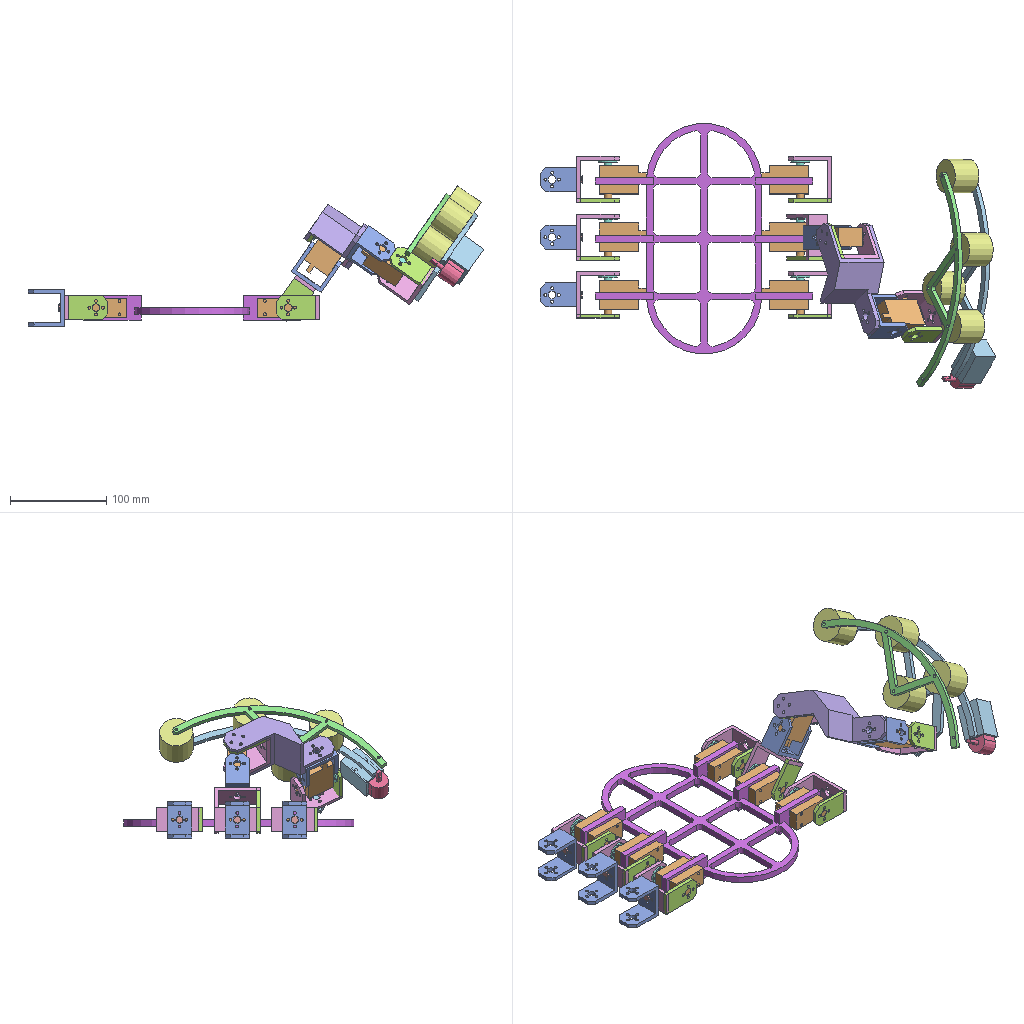Assembly | NX | 10 different items | 33 placed | box 474 x 275 x 146 mm
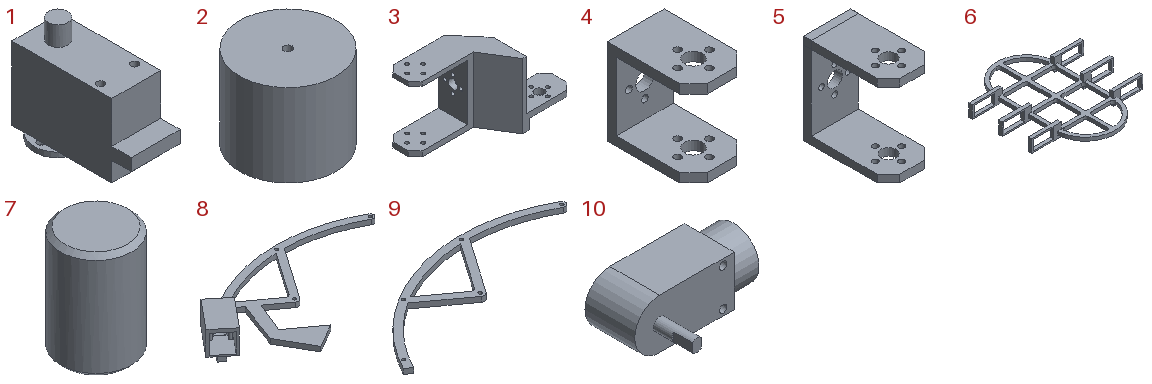Parts list (item | quantity | size | volume | features):
1 | x8 | 20 x 50 x 43 mm | 26482 mm3 | features DATUM_CSYS 6, EXTRUDE 6, SKETCH 5, MOVE_FACE 2
2 | x4 | 35 x 35 x 30 mm | 28651 mm3 | features DATUM_CSYS 2, EXTRUDE 1, HOLE PACKAGE 1, SIMPLE HOLE 1, SKETCH 1
3 | x1 | 110.372 x 51.171 x 56 mm | 51475 mm3 | features DATUM_CSYS 11, EXTRUDE 11, SKETCH 10, CHAMFER 2, MOVE_FACE 2
4 | x5 | 25 x 38 x 38 mm | 9370 mm3 | features DATUM_CSYS 4, MOVE_FACE 4, EXTRUDE 3, SKETCH 3, EXTRACT_BODY 2, EXTRACT_FACE 2, EXTRACT_STRING 2, Instance Feature 1, Mirror Feature 1, Pattern Geometry 1, REPLACE_FACE 1, UNITE 1
5 | x8 | 25 x 45 x 48 mm | 12170 mm3 | features DATUM_CSYS 4, EXTRUDE 3, MOVE_FACE 3, SKETCH 3, EXTRACT_BODY 2, EXTRACT_FACE 2, EXTRACT_STRING 2, Instance Feature 1, Mirror Feature 1, Pattern Geometry 1
6 | x1 | 226 x 240 x 26 mm | 84964 mm3 | features DATUM_CSYS 4, EXTRUDE 3, SKETCH 3, BLEND 1
7 | x3 | 8 x 8 x 12 mm | 597.164 mm3 | features CHAMFER 1, CYLINDER 1, DATUM_CSYS 1
8 | x1 | 216.068 x 114.552 x 30 mm | 29332 mm3 | features DATUM_CSYS 4, EXTRUDE 3, SKETCH 3, LINKED_BODY 1, MOVE_FACE 1, SUBTRACT 1
9 | x1 | 217.906 x 88.132 x 5 mm | 12489 mm3 | features DATUM_CSYS 3, EXTRUDE 2, SKETCH 2, MOVE_FACE 1
10 | x1 | 50 x 35 x 20 mm | 18267 mm3 | features DATUM_CSYS 5, SKETCH 4, EXTRUDE 3, BLEND 2, SIMPLE HOLE 2, BLOCK 1, HOLE PACKAGE 1, SCALE 1
Mates (type | each side: item.copy, entity, surface, feature):
Fix | 6.1 component
Touch | 1.1 face plane Extrude(2) | 6.1 face plane Extrude(3) | 11 times
Touch | 1.1 face plane Extrude(7) | 6.1 face plane Extrude(2) | 6 times
Concentric | 5.1 edge | 1.1 edge | 7 times
Touch | 6.1 face plane Extrude(3) | 1.1 face plane Extrude(2)
Concentric | 8.1 edge | 2.1 edge
Touch | 2.1 face cylinder Extrude(1) | 8.1 face cylinder Extrude(1)
Concentric | 9.1 edge | 2.1 edge
Touch | 9.1 face cylinder Extrude(1) | 2.1 face cylinder Extrude(1)
Concentric | 4.1 edge | 5.1 edge | 3 times
Touch | 1.1 face plane Extrude(2) | 4.1 face plane Mirror Feature(3)
Touch | 4.1 face cylinder Extrude(5) | 5.1 face cylinder Extrude(5) | 3 times
Touch | 5.1 face cylinder Mirror Feature(3) | 1.1 face cylinder Extrude(6)
Touch | 5.1 face plane Mirror Feature(3) | 1.1 face plane Extrude(6)
Touch | 3.1 face plane Extrude(3) | 5.1 face plane Extrude(2) | 2 times
Touch | 5.1 face plane Extrude(2) | 3.1 face plane Extrude(1)
Distance | 4.1 face plane Extrude(5) | 1.1 face plane Extrude(7)
Touch | 4.1 face cylinder Extrude(2) | 1.1 face cylinder Extrude(11) | 2 times
Touch | 1.1 face cylinder Extrude(11) | 4.1 face cylinder Extrude(2)
Concentric | 1.1 edge | 4.1 edge
Concentric | 4.1 edge | 3.1 edge
Touch | 4.1 face cylinder Extrude(5) | 3.1 face cylinder Extrude(13)
Touch | 8.1 face plane Linked Body(4) | 10.1 face plane Extrude(4)
Concentric | 2.1 edge | 9.1 edge
Touch | 10.1 face plane Block(1) | 8.1 face plane Linked Body(4) | 2 times
Concentric | 2.1 edge | 8.1 edge | 2 times
Touch | 8.1 face plane Extrude(1) | 5.1 face plane Extrude(2)
Touch | 5.1 face cylinder Extrude(5) | 4.1 face cylinder Extrude(5)
Concentric | 5.1 edge | 4.1 edge
Touch | 7.1 face cylinder Cylinder(1) | 4.1 face cylinder Extrude(5)
Distance | 7.1 face plane Cylinder(1) | 4.1 face plane Extrude(5)
Fix | assembly component
Bond | 7.1 component | assembly component | 3 times
LinearPattern | assembly axis | assembly csys | assembly csys | assembly csys